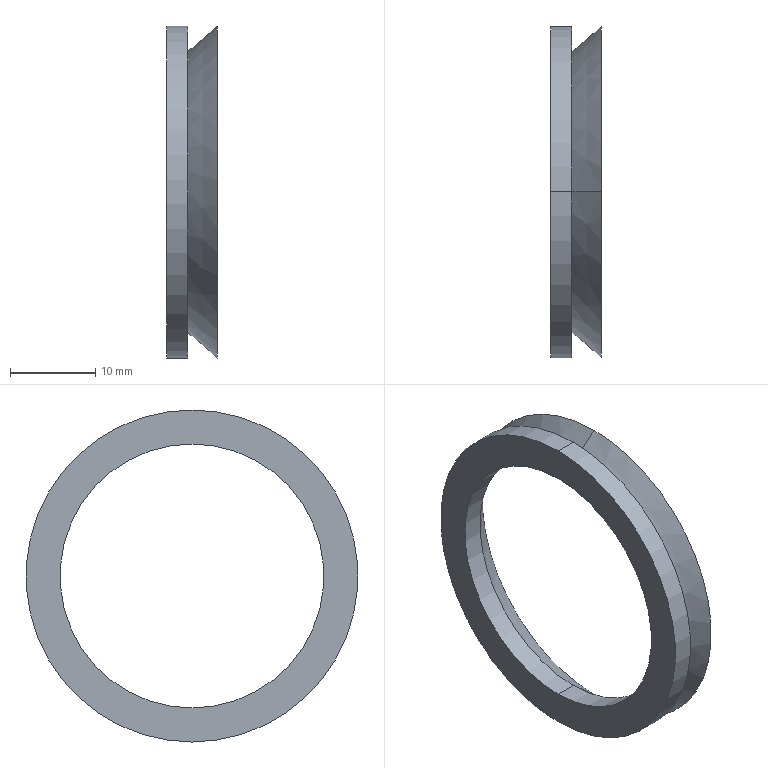Part | SolidWorks | features Revolution 1 | 1 solid | 11 faces | box 5.951 x 39 x 39 mm | volume 1479 mm3 | cylinder 4 | cone 4 | plane 3 | commonest cylinder face diameters 31 x2 39 x2
STEP:
#1=CARTESIAN_POINT('',(2.5,-15.5,-15.5));
#2=VERTEX_POINT('',#1);
#3=CARTESIAN_POINT('',(2.5,-15.5,15.5));
#4=VERTEX_POINT('',#3);
#5=CARTESIAN_POINT('',(2.5,-15.5,0.));
#6=DIRECTION('',(-1.,0.,0.));
#7=DIRECTION('',(0.,0.,1.));
#8=AXIS2_PLACEMENT_3D('',#5,#6,#7);
#9=CIRCLE('',#8,15.5);
#10=EDGE_CURVE('',#2,#4,#9,.T.);
#11=ORIENTED_EDGE('',*,*,#10,.F.);
#12=CARTESIAN_POINT('',(0.,-15.5,-15.5));
#13=VERTEX_POINT('',#12);
#14=CARTESIAN_POINT('',(-6.87,-15.5,-15.5));
#15=DIRECTION('',(-1.,0.,0.));
#16=VECTOR('',#15,1000.);
#17=LINE('',#14,#16);
#18=EDGE_CURVE('',#2,#13,#17,.T.);
#19=ORIENTED_EDGE('',*,*,#18,.T.);
#20=CARTESIAN_POINT('',(0.,-15.5,15.5));
#21=VERTEX_POINT('',#20);
#22=CARTESIAN_POINT('',(0.,-15.5,0.));
#23=DIRECTION('',(-1.,0.,0.));
#24=DIRECTION('',(0.,0.,1.));
#25=AXIS2_PLACEMENT_3D('',#22,#23,#24);
#26=CIRCLE('',#25,15.5);
#27=EDGE_CURVE('',#13,#21,#26,.T.);
#28=ORIENTED_EDGE('',*,*,#27,.T.);
#29=CARTESIAN_POINT('',(-6.87,-15.5,15.5));
#30=DIRECTION('',(-1.,0.,0.));
#31=VECTOR('',#30,1000.);
#32=LINE('',#29,#31);
#33=EDGE_CURVE('',#4,#21,#32,.T.);
#34=ORIENTED_EDGE('',*,*,#33,.F.);
#35=EDGE_LOOP('',(#11,#19,#28,#34));
#36=FACE_OUTER_BOUND('',#35,.T.);
#37=CARTESIAN_POINT('',(-6.87,-15.5,0.));
#38=DIRECTION('',(-1.,0.,0.));
#39=DIRECTION('',(0.,0.,1.));
#40=AXIS2_PLACEMENT_3D('',#37,#38,#39);
#41=CYLINDRICAL_SURFACE('',#40,15.5);
#42=ADVANCED_FACE('',(#36),#41,.F.);
#43=ORIENTED_EDGE('',*,*,#10,.T.);
#44=CARTESIAN_POINT('',(5.951,-15.5,18.5));
#45=VERTEX_POINT('',#44);
#46=CARTESIAN_POINT('',(2.5,-15.5,15.5));
#47=DIRECTION('',(0.7547,0.,0.6561));
#48=VECTOR('',#47,1000.);
#49=LINE('',#46,#48);
#50=EDGE_CURVE('',#4,#45,#49,.T.);
#51=ORIENTED_EDGE('',*,*,#50,.T.);
#52=CARTESIAN_POINT('',(5.951,-15.5,-18.5));
#53=VERTEX_POINT('',#52);
#54=CARTESIAN_POINT('',(5.951,-15.5,0.));
#55=DIRECTION('',(-1.,0.,0.));
#56=DIRECTION('',(0.,0.,1.));
#57=AXIS2_PLACEMENT_3D('',#54,#55,#56);
#58=CIRCLE('',#57,18.5);
#59=EDGE_CURVE('',#53,#45,#58,.T.);
#60=ORIENTED_EDGE('',*,*,#59,.F.);
#61=CARTESIAN_POINT('',(2.5,-15.5,-15.5));
#62=DIRECTION('',(0.7547,0.,-0.6561));
#63=VECTOR('',#62,1000.);
#64=LINE('',#61,#63);
#65=EDGE_CURVE('',#2,#53,#64,.T.);
#66=ORIENTED_EDGE('',*,*,#65,.F.);
#67=EDGE_LOOP('',(#43,#51,#60,#66));
#68=FACE_OUTER_BOUND('',#67,.T.);
#69=CARTESIAN_POINT('',(2.5,-15.5,0.));
#70=DIRECTION('',(1.,0.,0.));
#71=DIRECTION('',(0.,0.,-1.));
#72=AXIS2_PLACEMENT_3D('',#69,#70,#71);
#73=CONICAL_SURFACE('',#72,15.5,0.7156);
#74=ADVANCED_FACE('',(#68),#73,.F.);
#75=CARTESIAN_POINT('',(2.5,-15.5,16.5));
#76=VERTEX_POINT('',#75);
#77=CARTESIAN_POINT('',(2.5,-15.5,-16.5));
#78=VERTEX_POINT('',#77);
#79=CARTESIAN_POINT('',(2.5,-15.5,0.));
#80=DIRECTION('',(-1.,0.,0.));
#81=DIRECTION('',(0.,0.,1.));
#82=AXIS2_PLACEMENT_3D('',#79,#80,#81);
#83=CIRCLE('',#82,16.5);
#84=EDGE_CURVE('',#76,#78,#83,.T.);
#85=ORIENTED_EDGE('',*,*,#84,.F.);
#86=CARTESIAN_POINT('',(5.951,-15.5,19.5));
#87=VERTEX_POINT('',#86);
#88=CARTESIAN_POINT('',(5.951,-15.5,19.5));
#89=DIRECTION('',(0.7547,0.,0.6561));
#90=VECTOR('',#89,1000.);
#91=LINE('',#88,#90);
#92=EDGE_CURVE('',#76,#87,#91,.T.);
#93=ORIENTED_EDGE('',*,*,#92,.T.);
#94=CARTESIAN_POINT('',(5.951,-15.5,-19.5));
#95=VERTEX_POINT('',#94);
#96=CARTESIAN_POINT('',(5.951,-15.5,0.));
#97=DIRECTION('',(-1.,0.,0.));
#98=DIRECTION('',(0.,0.,1.));
#99=AXIS2_PLACEMENT_3D('',#96,#97,#98);
#100=CIRCLE('',#99,19.5);
#101=EDGE_CURVE('',#87,#95,#100,.T.);
#102=ORIENTED_EDGE('',*,*,#101,.T.);
#103=CARTESIAN_POINT('',(5.951,-15.5,-19.5));
#104=DIRECTION('',(0.7547,0.,-0.6561));
#105=VECTOR('',#104,1000.);
#106=LINE('',#103,#105);
#107=EDGE_CURVE('',#78,#95,#106,.T.);
#108=ORIENTED_EDGE('',*,*,#107,.F.);
#109=EDGE_LOOP('',(#85,#93,#102,#108));
#110=FACE_OUTER_BOUND('',#109,.T.);
#111=CARTESIAN_POINT('',(5.951,-15.5,0.));
#112=DIRECTION('',(1.,0.,0.));
#113=DIRECTION('',(0.,0.,-1.));
#114=AXIS2_PLACEMENT_3D('',#111,#112,#113);
#115=CONICAL_SURFACE('',#114,19.5,0.7156);
#116=ADVANCED_FACE('',(#110),#115,.T.);
#117=CARTESIAN_POINT('',(2.5,-15.5,19.5));
#118=VERTEX_POINT('',#117);
#119=CARTESIAN_POINT('',(2.5,-15.5,-19.5));
#120=VERTEX_POINT('',#119);
#121=CARTESIAN_POINT('',(2.5,-15.5,0.));
#122=DIRECTION('',(-1.,0.,0.));
#123=DIRECTION('',(0.,0.,1.));
#124=AXIS2_PLACEMENT_3D('',#121,#122,#123);
#125=CIRCLE('',#124,19.5);
#126=EDGE_CURVE('',#118,#120,#125,.T.);
#127=ORIENTED_EDGE('',*,*,#126,.T.);
#128=CARTESIAN_POINT('',(0.,-15.5,-19.5));
#129=VERTEX_POINT('',#128);
#130=CARTESIAN_POINT('',(-6.87,-15.5,-19.5));
#131=DIRECTION('',(-1.,0.,0.));
#132=VECTOR('',#131,1000.);
#133=LINE('',#130,#132);
#134=EDGE_CURVE('',#120,#129,#133,.T.);
#135=ORIENTED_EDGE('',*,*,#134,.T.);
#136=CARTESIAN_POINT('',(0.,-15.5,19.5));
#137=VERTEX_POINT('',#136);
#138=CARTESIAN_POINT('',(0.,-15.5,0.));
#139=DIRECTION('',(-1.,0.,0.));
#140=DIRECTION('',(0.,0.,1.));
#141=AXIS2_PLACEMENT_3D('',#138,#139,#140);
#142=CIRCLE('',#141,19.5);
#143=EDGE_CURVE('',#137,#129,#142,.T.);
#144=ORIENTED_EDGE('',*,*,#143,.F.);
#145=CARTESIAN_POINT('',(-6.87,-15.5,19.5));
#146=DIRECTION('',(-1.,0.,0.));
#147=VECTOR('',#146,1000.);
#148=LINE('',#145,#147);
#149=EDGE_CURVE('',#118,#137,#148,.T.);
#150=ORIENTED_EDGE('',*,*,#149,.F.);
#151=EDGE_LOOP('',(#127,#135,#144,#150));
#152=FACE_OUTER_BOUND('',#151,.T.);
#153=CARTESIAN_POINT('',(-6.87,-15.5,0.));
#154=DIRECTION('',(-1.,0.,0.));
#155=DIRECTION('',(0.,0.,1.));
#156=AXIS2_PLACEMENT_3D('',#153,#154,#155);
#157=CYLINDRICAL_SURFACE('',#156,19.5);
#158=ADVANCED_FACE('',(#152),#157,.T.);
#159=CARTESIAN_POINT('',(0.,-15.5,0.));
#160=DIRECTION('',(-1.,0.,0.));
#161=DIRECTION('',(0.,0.,1.));
#162=AXIS2_PLACEMENT_3D('',#159,#160,#161);
#163=CIRCLE('',#162,15.5);
#164=EDGE_CURVE('',#21,#13,#163,.T.);
#165=ORIENTED_EDGE('',*,*,#164,.F.);
#166=ORIENTED_EDGE('',*,*,#27,.F.);
#167=EDGE_LOOP('',(#165,#166));
#168=FACE_BOUND('',#167,.T.);
#169=ORIENTED_EDGE('',*,*,#143,.T.);
#170=CARTESIAN_POINT('',(0.,-15.5,0.));
#171=DIRECTION('',(-1.,0.,0.));
#172=DIRECTION('',(0.,0.,1.));
#173=AXIS2_PLACEMENT_3D('',#170,#171,#172);
#174=CIRCLE('',#173,19.5);
#175=EDGE_CURVE('',#129,#137,#174,.T.);
#176=ORIENTED_EDGE('',*,*,#175,.T.);
#177=EDGE_LOOP('',(#169,#176));
#178=FACE_OUTER_BOUND('',#177,.T.);
#179=CARTESIAN_POINT('',(0.,0.,0.));
#180=DIRECTION('',(1.,0.,0.));
#181=DIRECTION('',(0.,0.,-1.));
#182=AXIS2_PLACEMENT_3D('',#179,#180,#181);
#183=PLANE('',#182);
#184=ADVANCED_FACE('',(#168,#178),#183,.F.);
#185=ORIENTED_EDGE('',*,*,#134,.F.);
#186=CARTESIAN_POINT('',(2.5,-15.5,0.));
#187=DIRECTION('',(-1.,0.,0.));
#188=DIRECTION('',(0.,0.,1.));
#189=AXIS2_PLACEMENT_3D('',#186,#187,#188);
#190=CIRCLE('',#189,19.5);
#191=EDGE_CURVE('',#120,#118,#190,.T.);
#192=ORIENTED_EDGE('',*,*,#191,.T.);
#193=ORIENTED_EDGE('',*,*,#149,.T.);
#194=ORIENTED_EDGE('',*,*,#175,.F.);
#195=EDGE_LOOP('',(#185,#192,#193,#194));
#196=FACE_OUTER_BOUND('',#195,.T.);
#197=CARTESIAN_POINT('',(-6.87,-15.5,0.));
#198=DIRECTION('',(-1.,0.,0.));
#199=DIRECTION('',(0.,0.,1.));
#200=AXIS2_PLACEMENT_3D('',#197,#198,#199);
#201=CYLINDRICAL_SURFACE('',#200,19.5);
#202=ADVANCED_FACE('',(#196),#201,.T.);
#203=ORIENTED_EDGE('',*,*,#126,.F.);
#204=ORIENTED_EDGE('',*,*,#191,.F.);
#205=EDGE_LOOP('',(#203,#204));
#206=FACE_OUTER_BOUND('',#205,.T.);
#207=CARTESIAN_POINT('',(2.5,-15.5,0.));
#208=DIRECTION('',(-1.,0.,0.));
#209=DIRECTION('',(0.,0.,1.));
#210=AXIS2_PLACEMENT_3D('',#207,#208,#209);
#211=CIRCLE('',#210,16.5);
#212=EDGE_CURVE('',#78,#76,#211,.T.);
#213=ORIENTED_EDGE('',*,*,#212,.T.);
#214=ORIENTED_EDGE('',*,*,#84,.T.);
#215=EDGE_LOOP('',(#213,#214));
#216=FACE_BOUND('',#215,.T.);
#217=CARTESIAN_POINT('',(2.5,4.,0.));
#218=DIRECTION('',(-1.,0.,0.));
#219=DIRECTION('',(0.,0.,1.));
#220=AXIS2_PLACEMENT_3D('',#217,#218,#219);
#221=PLANE('',#220);
#222=ADVANCED_FACE('',(#206,#216),#221,.F.);
#223=ORIENTED_EDGE('',*,*,#92,.F.);
#224=ORIENTED_EDGE('',*,*,#212,.F.);
#225=ORIENTED_EDGE('',*,*,#107,.T.);
#226=CARTESIAN_POINT('',(5.951,-15.5,0.));
#227=DIRECTION('',(-1.,0.,0.));
#228=DIRECTION('',(0.,0.,1.));
#229=AXIS2_PLACEMENT_3D('',#226,#227,#228);
#230=CIRCLE('',#229,19.5);
#231=EDGE_CURVE('',#95,#87,#230,.T.);
#232=ORIENTED_EDGE('',*,*,#231,.T.);
#233=EDGE_LOOP('',(#223,#224,#225,#232));
#234=FACE_OUTER_BOUND('',#233,.T.);
#235=CARTESIAN_POINT('',(5.951,-15.5,0.));
#236=DIRECTION('',(1.,0.,0.));
#237=DIRECTION('',(0.,0.,-1.));
#238=AXIS2_PLACEMENT_3D('',#235,#236,#237);
#239=CONICAL_SURFACE('',#238,19.5,0.7156);
#240=ADVANCED_FACE('',(#234),#239,.T.);
#241=ORIENTED_EDGE('',*,*,#231,.F.);
#242=ORIENTED_EDGE('',*,*,#101,.F.);
#243=EDGE_LOOP('',(#241,#242));
#244=FACE_OUTER_BOUND('',#243,.T.);
#245=ORIENTED_EDGE('',*,*,#59,.T.);
#246=CARTESIAN_POINT('',(5.951,-15.5,0.));
#247=DIRECTION('',(-1.,0.,0.));
#248=DIRECTION('',(0.,0.,1.));
#249=AXIS2_PLACEMENT_3D('',#246,#247,#248);
#250=CIRCLE('',#249,18.5);
#251=EDGE_CURVE('',#45,#53,#250,.T.);
#252=ORIENTED_EDGE('',*,*,#251,.T.);
#253=EDGE_LOOP('',(#245,#252));
#254=FACE_BOUND('',#253,.T.);
#255=CARTESIAN_POINT('',(5.951,4.,0.));
#256=DIRECTION('',(-1.,0.,0.));
#257=DIRECTION('',(0.,0.,1.));
#258=AXIS2_PLACEMENT_3D('',#255,#256,#257);
#259=PLANE('',#258);
#260=ADVANCED_FACE('',(#244,#254),#259,.F.);
#261=ORIENTED_EDGE('',*,*,#50,.F.);
#262=CARTESIAN_POINT('',(2.5,-15.5,0.));
#263=DIRECTION('',(-1.,0.,0.));
#264=DIRECTION('',(0.,0.,1.));
#265=AXIS2_PLACEMENT_3D('',#262,#263,#264);
#266=CIRCLE('',#265,15.5);
#267=EDGE_CURVE('',#4,#2,#266,.T.);
#268=ORIENTED_EDGE('',*,*,#267,.T.);
#269=ORIENTED_EDGE('',*,*,#65,.T.);
#270=ORIENTED_EDGE('',*,*,#251,.F.);
#271=EDGE_LOOP('',(#261,#268,#269,#270));
#272=FACE_OUTER_BOUND('',#271,.T.);
#273=CARTESIAN_POINT('',(2.5,-15.5,0.));
#274=DIRECTION('',(1.,0.,0.));
#275=DIRECTION('',(0.,0.,-1.));
#276=AXIS2_PLACEMENT_3D('',#273,#274,#275);
#277=CONICAL_SURFACE('',#276,15.5,0.7156);
#278=ADVANCED_FACE('',(#272),#277,.F.);
#279=ORIENTED_EDGE('',*,*,#18,.F.);
#280=ORIENTED_EDGE('',*,*,#267,.F.);
#281=ORIENTED_EDGE('',*,*,#33,.T.);
#282=ORIENTED_EDGE('',*,*,#164,.T.);
#283=EDGE_LOOP('',(#279,#280,#281,#282));
#284=FACE_OUTER_BOUND('',#283,.T.);
#285=CARTESIAN_POINT('',(-6.87,-15.5,0.));
#286=DIRECTION('',(-1.,0.,0.));
#287=DIRECTION('',(0.,0.,1.));
#288=AXIS2_PLACEMENT_3D('',#285,#286,#287);
#289=CYLINDRICAL_SURFACE('',#288,15.5);
#290=ADVANCED_FACE('',(#284),#289,.F.);
#291=CLOSED_SHELL('',(#42,#74,#116,#158,#184,#202,#222,#240,#260,#278,#290));
#292=MANIFOLD_SOLID_BREP('',#291);
#293=CARTESIAN_POINT('',(0.,0.,0.));
#294=DIRECTION('',(0.,0.,1.));
#295=DIRECTION('',(1.,0.,0.));
#296=AXIS2_PLACEMENT_3D('',#293,#294,#295);
#297=(LENGTH_UNIT()NAMED_UNIT(*)SI_UNIT(.MILLI.,.METRE.));
#298=UNCERTAINTY_MEASURE_WITH_UNIT(LENGTH_MEASURE(0.00001),#297,'','');
#299=(NAMED_UNIT(*)PLANE_ANGLE_UNIT()SI_UNIT($,.RADIAN.));
#300=(NAMED_UNIT(*)SI_UNIT($,.STERADIAN.)SOLID_ANGLE_UNIT());
#301=(GEOMETRIC_REPRESENTATION_CONTEXT(3)GLOBAL_UNCERTAINTY_ASSIGNED_CONTEXT((#298))GLOBAL_UNIT_ASSIGNED_CONTEXT((#297,#299,#300))REPRESENTATION_CONTEXT('',''));
#302=ADVANCED_BREP_SHAPE_REPRESENTATION('',(#292,#296),#301);